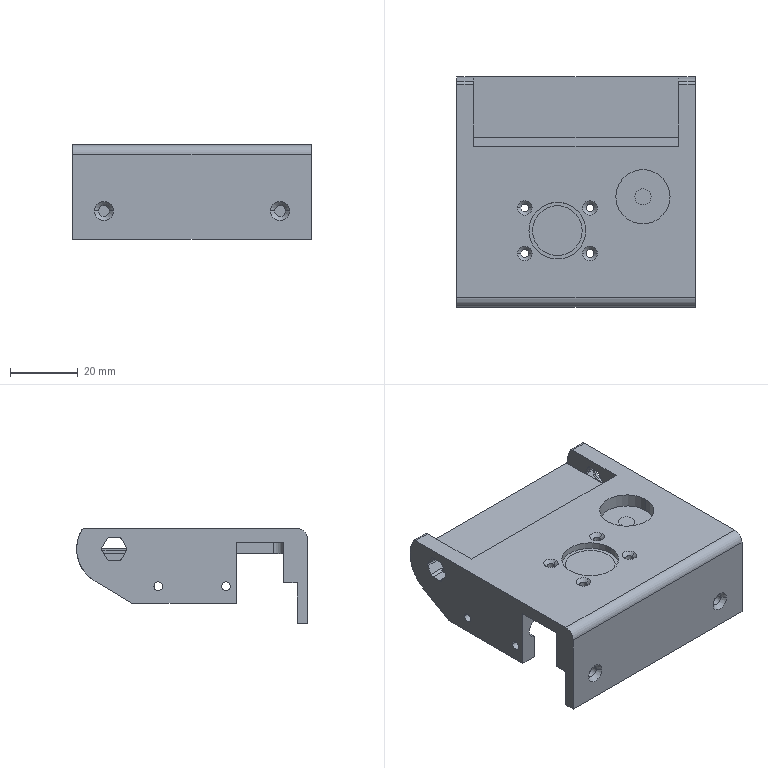NC program | NX | posted with a generic post | part box 70.5 x 68.1 x 28 mm
Lines 2811 to 2864 of 2864:
(ZLEVEL_PROFILE_1_COPY_1_COPY_COPY_COPY_1_COPY_COPY_COPY , TOOL : D6A45)
N5596 T07 M6
N5598 G54
N5600 G17 G0 G90 X50. Y-18.841 B0. C0. S9500 M3
N5602 G43 Z30. H7
N5604 Z1.
N5606 G94 G1 Z-1. F1000.
N5608 G3 X50.341 Y-18.5 R0.341
N5610 X50. Y-18.841 R-0.341
N5612 X50.26 Y-18.691 R0.3
N5614 G1 Z0.
N5616 G0 Z30.
N5618 X5. Y-4.709
N5620 Z1.
N5622 G1 Z-1.
N5624 G3 X4.709 Y-5. R0.291
N5626 X5. Y-4.709 R-0.291
N5628 X4.74 Y-4.859 R0.3
N5630 G1 Z0.
N5632 G0 Z30.
N5634 X58.439 Y-4.851
N5636 Z0.
N5638 G1 Z-1.
N5640 X57.52 Y-3.259
N5642 G3 X57. Y-2.959 R0.6
N5644 X53.959 Y-6. R3.041
N5646 X57. Y-2.959 R-3.041
N5648 X56.48 Y-3.259 R0.6
N5650 G1 X55.561 Y-4.851
N5652 Z0.
N5654 G0 Z30.
N5656 M5
(刀补4 , TOOL : D4)
N5658 T04 M6
N5660 G54
N5662 G17 G0 G90 X57.782 Y-4.7 B0. C0. S9500 M3
N5664 G43 Z30. H4
N5666 Z0.768
N5668 G94 G1 Z-0.732 F1000.
N5670 G41 X57.775 Y-4.6 D4
N5672 G3 X57. Y-4. R0.8
N5674 X55. Y-6. R2.
N5676 X57. Y-4. R-2.
N5678 X56.225 Y-4.6 R0.8
N5680 G40
N5682 G1 X56.218 Y-4.7
N5684 Z0.768
N5686 G0 Z30.
N5688 M5
N5690 M2